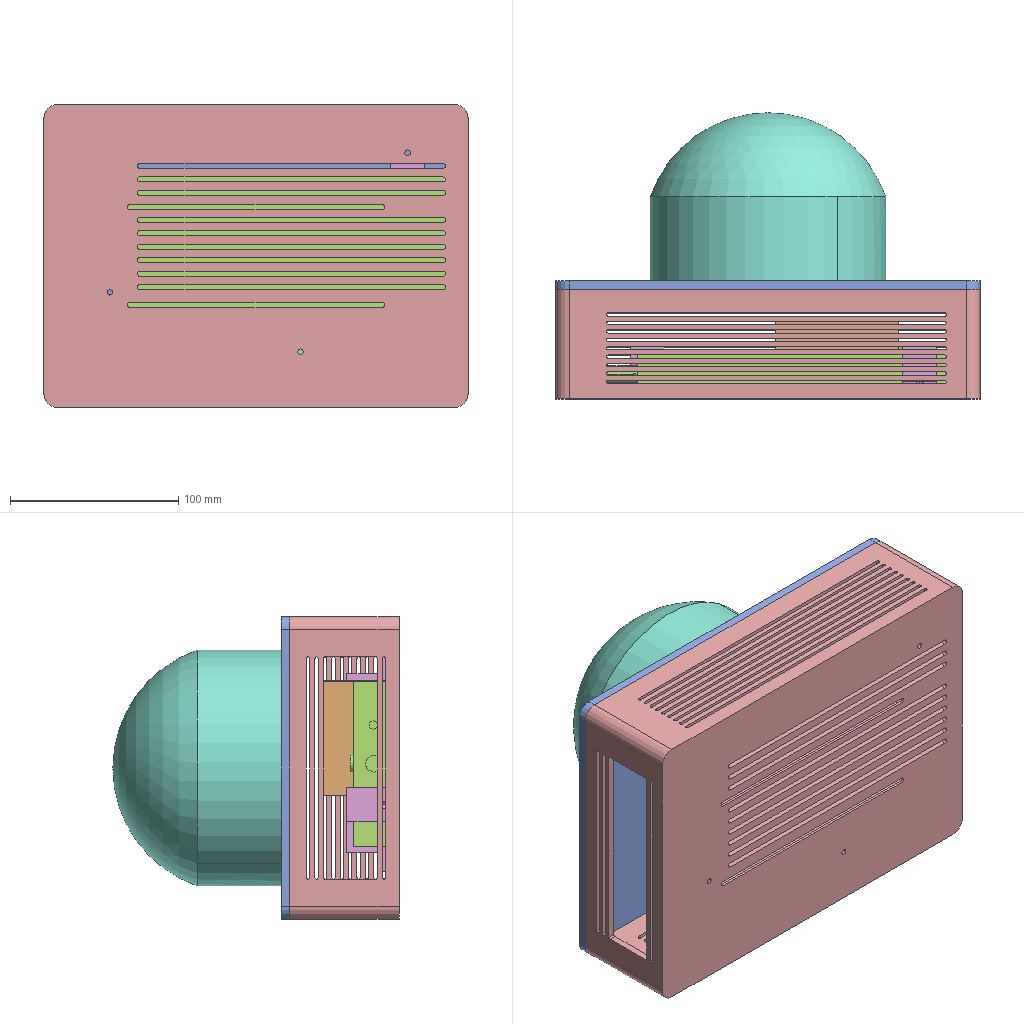Assembly | SolidWorks | 6 different items | 8 placed | box 252 x 170 x 180 mm
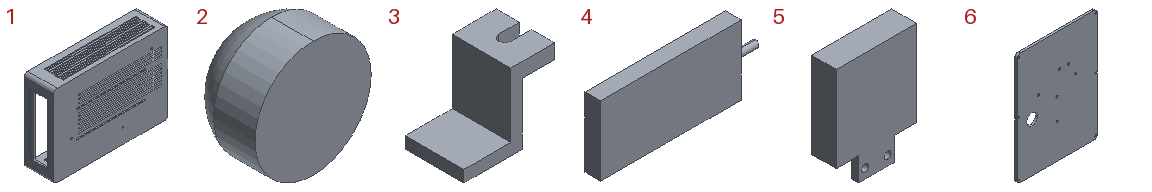Parts list (item | quantity | size | volume | features):
1 | x1 | 252 x 65 x 180 mm | 401045 mm3 | features ICE 11, Fillet 5, MoveFace 5, HoleWzd 2, Cut 1, Extrusion 1
2 | x1 | 140 x 100 x 140 mm | 1219985 mm3 | features Dome 1, Extrusion 1
3 | x3 | 31 x 20 x 26 mm | 4278 mm3 | features Extrusion 1, ICE 1
4 | x1 | 228 x 24 x 98 mm | 429480 mm3 | features ICE 3, Extrusion 1
5 | x1 | 68 x 21 x 93 mm | 107516 mm3 | features ICE 2, Extrusion 1
6 | x1 | 180 x 5 x 252 mm | 223279 mm3 | features ICE 5, HoleWzd 2, Dome 1, Extrusion 1, Fillet 1
Mates (type | each side: item.copy, entity, surface, feature):
Coincident | 1.1 face plane Boss-Extrude2 | 6.1 face plane Boss-Extrude1
Coincident | 1.1 face plane Boss-Extrude1 | 4.1 face plane Boss-Extrude1
Coincident | 1.1 face plane Boss-Extrude1 | 3.1 face plane Boss-Extrude1
Coincident | 4.1 face plane Boss-Extrude1 | 3.1 face plane Boss-Extrude1
Coincident | 1.1 face plane Boss-Extrude1 | 3.2 face plane Boss-Extrude1
Coincident | 1.1 face plane Boss-Extrude1 | 3.3 face plane Boss-Extrude1
Coincident | 4.1 face plane Boss-Extrude1 | 3.2 face plane Boss-Extrude1
Coincident | 4.1 face plane Boss-Extrude1 | 3.3 face plane Boss-Extrude1
Concentric | 1.1 face cylinder M3 Tapped Hole4 | 6.1 face cone CSK for M3 Flat Head Machine Screw1
Coincident | 6.1 face plane Boss-Extrude1 | 2.1 face plane Boss-Extrude1
Concentric | 6.1 face cylinder Cut-Extrude3 | 2.1 face cylinder Boss-Extrude1
Coincident | 4.1 face plane Boss-Extrude1 | 5.1 face plane Boss-Extrude1